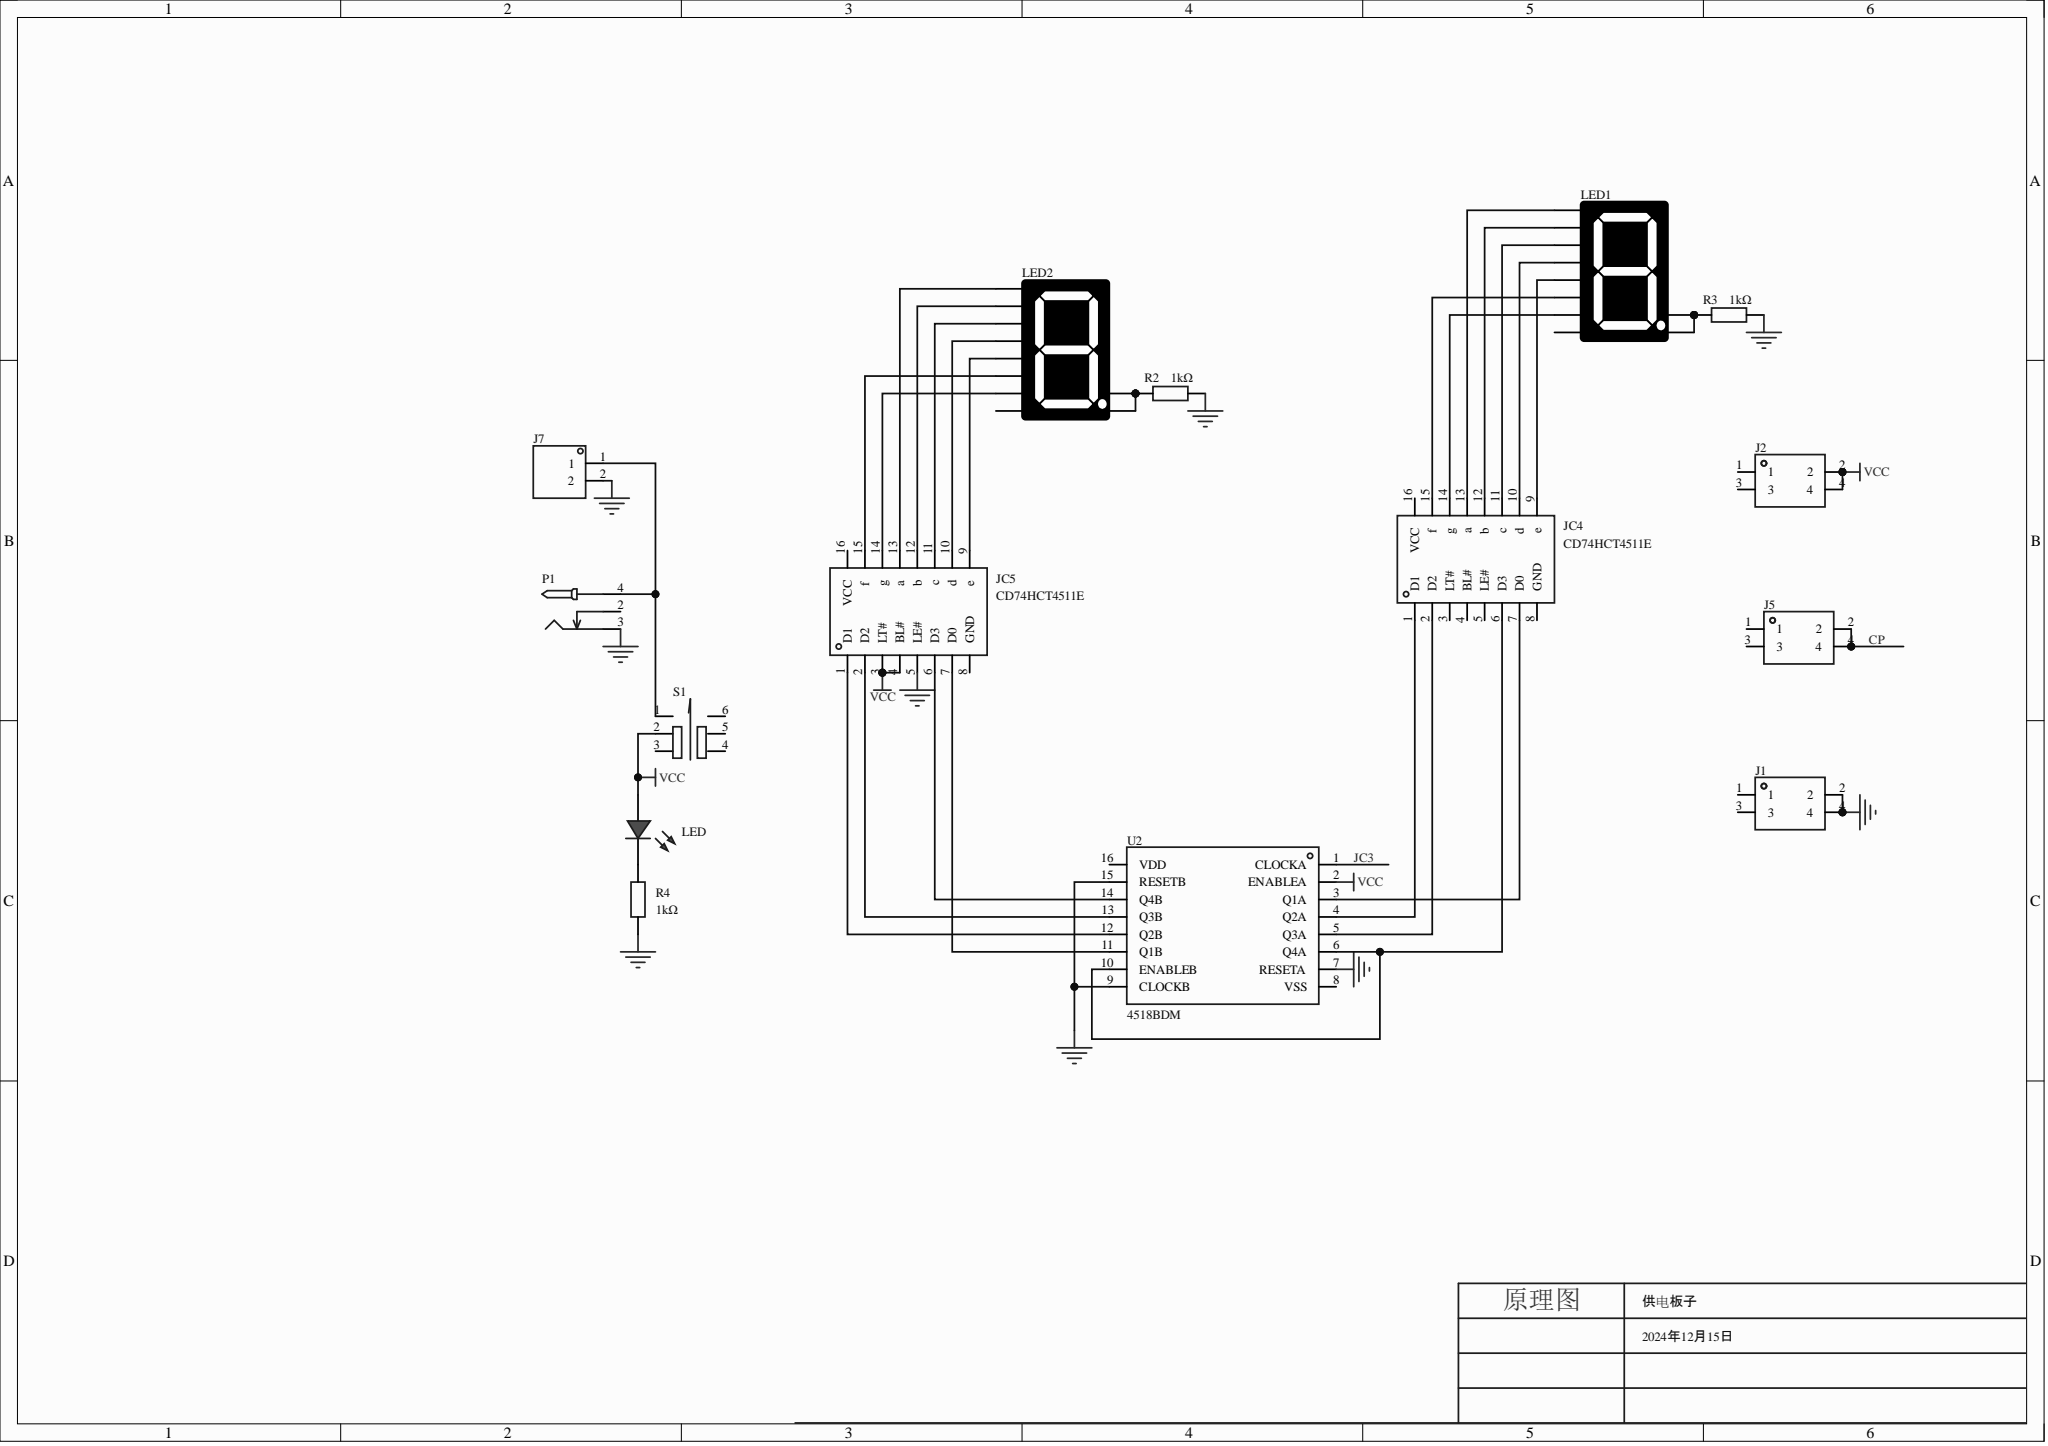Circuit board | Altium Designer | 15 parts | 29 nets
Bill of materials:
Comment,Description,Designator,Footprint,LibRef,Quantity
"","","J1, J2, J5","HDR-TH_4P-P2.54-V-M-R2-C2-S2.54-1","HDR-M_2.54_2x2","3"
"","","J7","HDR-TH_2P-P2.54-V-M-1","HDR-M_2.54_1x2P","1"
"CD74HCT4511E","高速 CMOS 逻辑 BCD 至 7 段锁存器/解码器/驱动器 16-PDIP -55 to 125","JC4, JC5","PDIP-16_L19.3-W6.4-P2.54-LS7.94-BL","CD74HCT4511E","2"
"","","LED","LED-TH_5mm","LED_TH-R_5mm","1"
"","","LED1, LED2","LED-SEG-TH_10P-L12.6-W19.0-P2.54-S15.24-BL","LED_SEG_TH_0.56x1","2"
"","","P1","DC-2.0","DC-005_2.0","1"
"1kΩ","","R2, R3, R4","Res_1/8W","Res_AXIAL-1/8W","3"
"自锁开关 5.8Z白灰白260G","耐温260度","S1","SW-TH_6P-L5.8-W5.8-P2.00-LS4.5-TR","自锁开关 5.8Z白灰白260G","1"
"4518BDM","工作电压:5V~15V;元件数:2;每个元件位数:4;触发器类型:正边沿；负边沿;计数速率:12MHz;","U2","PDIP-16_L19.3-W6.4-P2.54-LS7.94-BL","4518BDM","1"
Netlist (Protel format):
[
J1
HDR-TH_4P-P2.54-V-M-R2-C2-S2.54-1




]
[
J2
HDR-TH_4P-P2.54-V-M-R2-C2-S2.54-1




]
[
J5
HDR-TH_4P-P2.54-V-M-R2-C2-S2.54-1




]
[
J7
HDR-TH_2P-P2.54-V-M-1




]
[
JC4
PDIP-16_L19.3-W6.4-P2.54-LS7.94-BL
CD74HCT4511E



]
[
JC5
PDIP-16_L19.3-W6.4-P2.54-LS7.94-BL
CD74HCT4511E



]
[
LED
LED-TH_5mm




]
[
LED1
LED-SEG-TH_10P-L12.6-W19.0-P2.54-S15.24-BL




]
[
LED2
LED-SEG-TH_10P-L12.6-W19.0-P2.54-S15.24-BL




]
[
P1
DC-2.0




]
[
R2
Res_1/8W
1kΩ



]
[
R3
Res_1/8W
1kΩ



]
[
R4
Res_1/8W
1kΩ



]
[
S1
SW-TH_6P-L5.8-W5.8-P2.00-LS4.5-TR
自锁开关 5.8Z白灰白260G



]
[
U2
PDIP-16_L19.3-W6.4-P2.54-LS7.94-BL
4518BDM



]
(
VCC
J2-2
J2-4
JC5-3
JC5-4
LED-1
S1-2
U2-2
)
(
NetLED_2
LED-2
R4-2
)
(
NetLED2_3
LED2-3
LED2-8
R2-1
)
(
NetLED1_3
LED1-3
LED1-8
R3-1
)
(
NetJC5_15
JC5-15
LED2-9
)
(
NetJC5_14
JC5-14
LED2-10
)
(
NetJC5_13
JC5-13
LED2-7
)
(
NetJC5_12
JC5-12
LED2-6
)
(
NetJC5_11
JC5-11
LED2-4
)
(
NetJC5_10
JC5-10
LED2-2
)
(
NetJC5_9
JC5-9
LED2-1
)
(
NetJC5_7
JC5-7
U2-11
)
(
NetJC5_6
JC5-6
U2-14
)
(
NetJC5_2
JC5-2
U2-13
)
(
NetJC5_1
JC5-1
U2-12
)
(
NetJC4_15
JC4-15
LED1-9
)
(
NetJC4_14
JC4-14
LED1-10
)
(
NetJC4_13
JC4-13
LED1-7
)
(
NetJC4_12
JC4-12
LED1-6
)
(
NetJC4_11
JC4-11
LED1-4
)
(
NetJC4_10
JC4-10
LED1-2
)
(
NetJC4_9
JC4-9
LED1-1
)
(
NetJC4_7
JC4-7
U2-3
)
(
NetJC4_6
JC4-6
U2-6
U2-10
)
(
NetJC4_2
JC4-2
U2-5
)
(
NetJC4_1
JC4-1
U2-4
)
(
NetJ7_1
J7-1
P1-4
S1-1
)
(
GND
J1-2
J1-4
J7-2
JC5-5
P1-3
R2-2
R3-2
R4-1
U2-7
U2-9
U2-15
)
(
CP
J5-2
J5-4
)